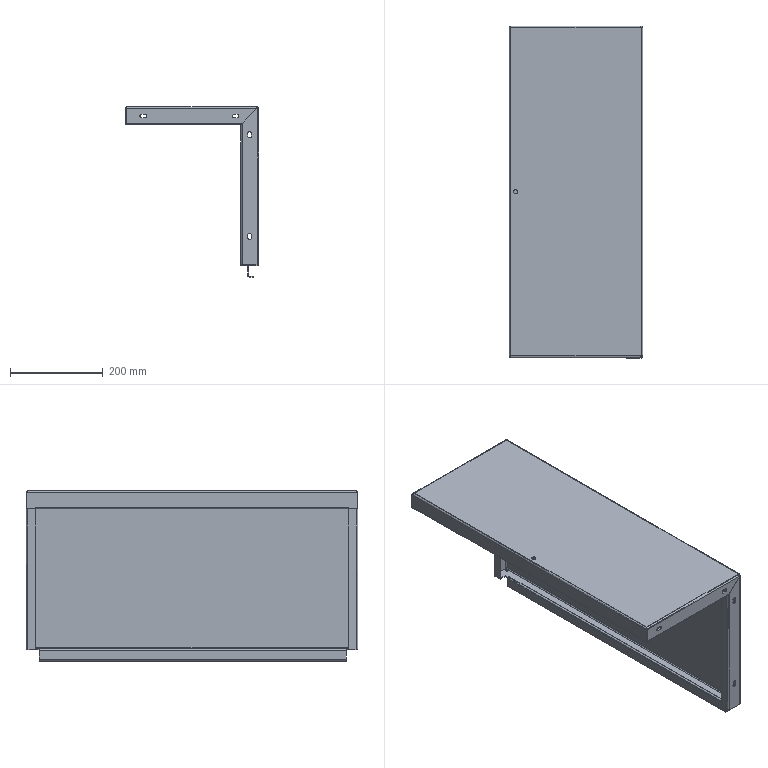Part | NX | features solid 2 | 1 solid | 172 faces | box 289.001 x 717 x 368.001 mm | volume 1167841 mm3 | plane 106 | cylinder 58 | spline 8 | commonest cylinder face diameters 8 x38 4 x14 3.8 x2 6.5 x2 9.2 x2